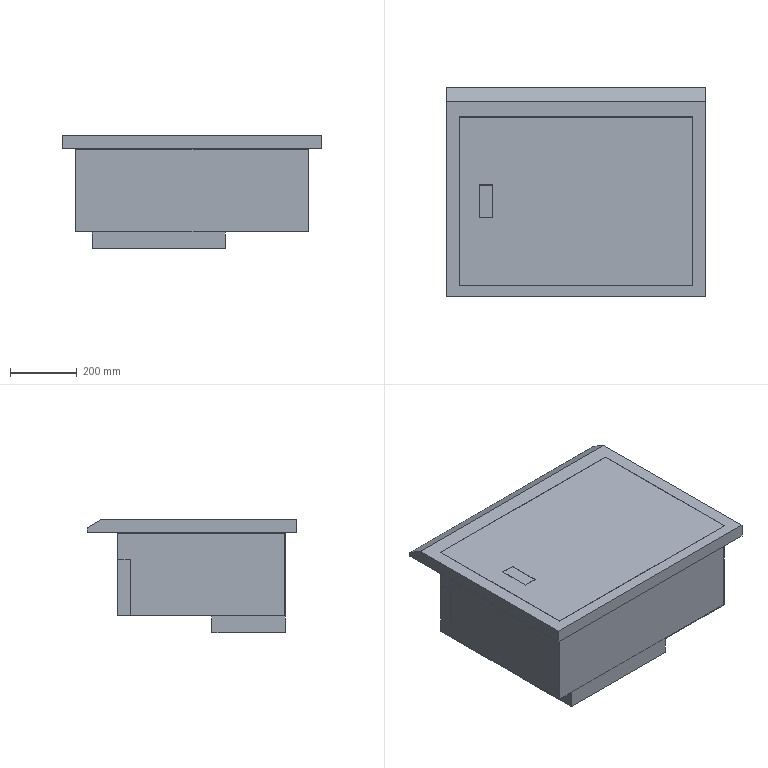Part | SolidWorks | features ICE 9, CutThin 1, Extrusion 1, Shell 1 | 1 solid | 50 faces | box 780 x 630 x 340 mm | volume 30091258 mm3 | plane 50
STEP:
#1=CARTESIAN_POINT('',(0.,505.,250.));
#2=VERTEX_POINT('',#1);
#3=CARTESIAN_POINT('',(0.,505.,0.));
#4=VERTEX_POINT('',#3);
#5=CARTESIAN_POINT('',(0.,505.,250.));
#6=DIRECTION('',(0.,0.,-1.));
#7=VECTOR('',#6,1000.);
#8=LINE('',#5,#7);
#9=EDGE_CURVE('',#2,#4,#8,.T.);
#10=ORIENTED_EDGE('',*,*,#9,.T.);
#11=CARTESIAN_POINT('',(0.,0.,0.));
#12=VERTEX_POINT('',#11);
#13=CARTESIAN_POINT('',(0.,0.,0.));
#14=DIRECTION('',(0.,-1.,0.));
#15=VECTOR('',#14,1000.);
#16=LINE('',#13,#15);
#17=EDGE_CURVE('',#4,#12,#16,.T.);
#18=ORIENTED_EDGE('',*,*,#17,.T.);
#19=CARTESIAN_POINT('',(0.,0.,250.));
#20=VERTEX_POINT('',#19);
#21=CARTESIAN_POINT('',(0.,0.,250.));
#22=DIRECTION('',(0.,0.,-1.));
#23=VECTOR('',#22,1000.);
#24=LINE('',#21,#23);
#25=EDGE_CURVE('',#20,#12,#24,.T.);
#26=ORIENTED_EDGE('',*,*,#25,.F.);
#27=CARTESIAN_POINT('',(0.,0.,250.));
#28=DIRECTION('',(0.,-1.,0.));
#29=VECTOR('',#28,1000.);
#30=LINE('',#27,#29);
#31=EDGE_CURVE('',#2,#20,#30,.T.);
#32=ORIENTED_EDGE('',*,*,#31,.F.);
#33=EDGE_LOOP('',(#10,#18,#26,#32));
#34=FACE_OUTER_BOUND('',#33,.T.);
#35=CARTESIAN_POINT('',(0.,0.,250.));
#36=DIRECTION('',(1.,0.,0.));
#37=DIRECTION('',(0.,0.,-1.));
#38=AXIS2_PLACEMENT_3D('',#35,#36,#37);
#39=PLANE('',#38);
#40=ADVANCED_FACE('',(#34),#39,.F.);
#41=ORIENTED_EDGE('',*,*,#25,.T.);
#42=CARTESIAN_POINT('',(50.,0.,0.));
#43=VERTEX_POINT('',#42);
#44=CARTESIAN_POINT('',(0.,0.,0.));
#45=DIRECTION('',(1.,0.,0.));
#46=VECTOR('',#45,1000.);
#47=LINE('',#44,#46);
#48=EDGE_CURVE('',#12,#43,#47,.T.);
#49=ORIENTED_EDGE('',*,*,#48,.T.);
#50=CARTESIAN_POINT('',(50.,0.,-50.));
#51=VERTEX_POINT('',#50);
#52=CARTESIAN_POINT('',(50.,0.,-50.));
#53=DIRECTION('',(0.,0.,1.));
#54=VECTOR('',#53,1000.);
#55=LINE('',#52,#54);
#56=EDGE_CURVE('',#51,#43,#55,.T.);
#57=ORIENTED_EDGE('',*,*,#56,.F.);
#58=CARTESIAN_POINT('',(450.,0.,-50.));
#59=VERTEX_POINT('',#58);
#60=CARTESIAN_POINT('',(50.,0.,-50.));
#61=DIRECTION('',(-1.,0.,0.));
#62=VECTOR('',#61,1000.);
#63=LINE('',#60,#62);
#64=EDGE_CURVE('',#59,#51,#63,.T.);
#65=ORIENTED_EDGE('',*,*,#64,.F.);
#66=CARTESIAN_POINT('',(450.,0.,0.));
#67=VERTEX_POINT('',#66);
#68=CARTESIAN_POINT('',(450.,0.,-50.));
#69=DIRECTION('',(0.,0.,1.));
#70=VECTOR('',#69,1000.);
#71=LINE('',#68,#70);
#72=EDGE_CURVE('',#59,#67,#71,.T.);
#73=ORIENTED_EDGE('',*,*,#72,.T.);
#74=CARTESIAN_POINT('',(700.,0.,0.));
#75=VERTEX_POINT('',#74);
#76=CARTESIAN_POINT('',(0.,0.,0.));
#77=DIRECTION('',(1.,0.,0.));
#78=VECTOR('',#77,1000.);
#79=LINE('',#76,#78);
#80=EDGE_CURVE('',#67,#75,#79,.T.);
#81=ORIENTED_EDGE('',*,*,#80,.T.);
#82=CARTESIAN_POINT('',(700.,0.,250.));
#83=VERTEX_POINT('',#82);
#84=CARTESIAN_POINT('',(700.,0.,250.));
#85=DIRECTION('',(0.,0.,-1.));
#86=VECTOR('',#85,1000.);
#87=LINE('',#84,#86);
#88=EDGE_CURVE('',#83,#75,#87,.T.);
#89=ORIENTED_EDGE('',*,*,#88,.F.);
#90=CARTESIAN_POINT('',(0.,0.,250.));
#91=DIRECTION('',(1.,0.,0.));
#92=VECTOR('',#91,1000.);
#93=LINE('',#90,#92);
#94=EDGE_CURVE('',#20,#83,#93,.T.);
#95=ORIENTED_EDGE('',*,*,#94,.F.);
#96=EDGE_LOOP('',(#41,#49,#57,#65,#73,#81,#89,#95));
#97=FACE_OUTER_BOUND('',#96,.T.);
#98=CARTESIAN_POINT('',(0.,0.,250.));
#99=DIRECTION('',(0.,1.,0.));
#100=DIRECTION('',(0.,0.,1.));
#101=AXIS2_PLACEMENT_3D('',#98,#99,#100);
#102=PLANE('',#101);
#103=ADVANCED_FACE('',(#97),#102,.F.);
#104=CARTESIAN_POINT('',(700.,505.,0.));
#105=VERTEX_POINT('',#104);
#106=CARTESIAN_POINT('',(700.,0.,0.));
#107=DIRECTION('',(0.,1.,0.));
#108=VECTOR('',#107,1000.);
#109=LINE('',#106,#108);
#110=EDGE_CURVE('',#75,#105,#109,.T.);
#111=ORIENTED_EDGE('',*,*,#110,.T.);
#112=CARTESIAN_POINT('',(700.,505.,250.));
#113=VERTEX_POINT('',#112);
#114=CARTESIAN_POINT('',(700.,505.,250.));
#115=DIRECTION('',(0.,0.,-1.));
#116=VECTOR('',#115,1000.);
#117=LINE('',#114,#116);
#118=EDGE_CURVE('',#113,#105,#117,.T.);
#119=ORIENTED_EDGE('',*,*,#118,.F.);
#120=CARTESIAN_POINT('',(700.,0.,250.));
#121=DIRECTION('',(0.,1.,0.));
#122=VECTOR('',#121,1000.);
#123=LINE('',#120,#122);
#124=EDGE_CURVE('',#83,#113,#123,.T.);
#125=ORIENTED_EDGE('',*,*,#124,.F.);
#126=ORIENTED_EDGE('',*,*,#88,.T.);
#127=EDGE_LOOP('',(#111,#119,#125,#126));
#128=FACE_OUTER_BOUND('',#127,.T.);
#129=CARTESIAN_POINT('',(700.,0.,250.));
#130=DIRECTION('',(-1.,0.,0.));
#131=DIRECTION('',(0.,0.,1.));
#132=AXIS2_PLACEMENT_3D('',#129,#130,#131);
#133=PLANE('',#132);
#134=ADVANCED_FACE('',(#128),#133,.F.);
#135=ORIENTED_EDGE('',*,*,#118,.T.);
#136=CARTESIAN_POINT('',(700.,505.,0.));
#137=DIRECTION('',(-1.,0.,0.));
#138=VECTOR('',#137,1000.);
#139=LINE('',#136,#138);
#140=EDGE_CURVE('',#105,#4,#139,.T.);
#141=ORIENTED_EDGE('',*,*,#140,.T.);
#142=ORIENTED_EDGE('',*,*,#9,.F.);
#143=CARTESIAN_POINT('',(0.,505.,250.));
#144=DIRECTION('',(-1.,0.,0.));
#145=VECTOR('',#144,1000.);
#146=LINE('',#143,#145);
#147=EDGE_CURVE('',#113,#2,#146,.T.);
#148=ORIENTED_EDGE('',*,*,#147,.F.);
#149=EDGE_LOOP('',(#135,#141,#142,#148));
#150=FACE_OUTER_BOUND('',#149,.T.);
#151=CARTESIAN_POINT('',(0.,505.,250.));
#152=DIRECTION('',(0.,-1.,0.));
#153=DIRECTION('',(0.,0.,-1.));
#154=AXIS2_PLACEMENT_3D('',#151,#152,#153);
#155=PLANE('',#154);
#156=ADVANCED_FACE('',(#150),#155,.F.);
#157=CARTESIAN_POINT('',(50.,220.,0.));
#158=VERTEX_POINT('',#157);
#159=CARTESIAN_POINT('',(50.,0.,0.));
#160=DIRECTION('',(0.,1.,0.));
#161=VECTOR('',#160,1000.);
#162=LINE('',#159,#161);
#163=EDGE_CURVE('',#43,#158,#162,.T.);
#164=ORIENTED_EDGE('',*,*,#163,.F.);
#165=ORIENTED_EDGE('',*,*,#48,.F.);
#166=ORIENTED_EDGE('',*,*,#17,.F.);
#167=ORIENTED_EDGE('',*,*,#140,.F.);
#168=ORIENTED_EDGE('',*,*,#110,.F.);
#169=ORIENTED_EDGE('',*,*,#80,.F.);
#170=CARTESIAN_POINT('',(450.,220.,0.));
#171=VERTEX_POINT('',#170);
#172=CARTESIAN_POINT('',(450.,0.,0.));
#173=DIRECTION('',(0.,-1.,0.));
#174=VECTOR('',#173,1000.);
#175=LINE('',#172,#174);
#176=EDGE_CURVE('',#171,#67,#175,.T.);
#177=ORIENTED_EDGE('',*,*,#176,.F.);
#178=CARTESIAN_POINT('',(50.,220.,0.));
#179=DIRECTION('',(1.,0.,0.));
#180=VECTOR('',#179,1000.);
#181=LINE('',#178,#180);
#182=EDGE_CURVE('',#158,#171,#181,.T.);
#183=ORIENTED_EDGE('',*,*,#182,.F.);
#184=EDGE_LOOP('',(#164,#165,#166,#167,#168,#169,#177,#183));
#185=FACE_OUTER_BOUND('',#184,.T.);
#186=CARTESIAN_POINT('',(0.,0.,0.));
#187=DIRECTION('',(0.,0.,-1.));
#188=DIRECTION('',(-1.,0.,0.));
#189=AXIS2_PLACEMENT_3D('',#186,#187,#188);
#190=PLANE('',#189);
#191=ADVANCED_FACE('',(#185),#190,.T.);
#192=ORIENTED_EDGE('',*,*,#163,.T.);
#193=CARTESIAN_POINT('',(50.,220.,-50.));
#194=VERTEX_POINT('',#193);
#195=CARTESIAN_POINT('',(50.,220.,-50.));
#196=DIRECTION('',(0.,0.,1.));
#197=VECTOR('',#196,1000.);
#198=LINE('',#195,#197);
#199=EDGE_CURVE('',#194,#158,#198,.T.);
#200=ORIENTED_EDGE('',*,*,#199,.F.);
#201=CARTESIAN_POINT('',(50.,0.,-50.));
#202=DIRECTION('',(0.,1.,0.));
#203=VECTOR('',#202,1000.);
#204=LINE('',#201,#203);
#205=EDGE_CURVE('',#51,#194,#204,.T.);
#206=ORIENTED_EDGE('',*,*,#205,.F.);
#207=ORIENTED_EDGE('',*,*,#56,.T.);
#208=EDGE_LOOP('',(#192,#200,#206,#207));
#209=FACE_OUTER_BOUND('',#208,.T.);
#210=CARTESIAN_POINT('',(50.,0.,-50.));
#211=DIRECTION('',(1.,0.,0.));
#212=DIRECTION('',(0.,1.,0.));
#213=AXIS2_PLACEMENT_3D('',#210,#211,#212);
#214=PLANE('',#213);
#215=ADVANCED_FACE('',(#209),#214,.F.);
#216=ORIENTED_EDGE('',*,*,#182,.T.);
#217=CARTESIAN_POINT('',(450.,220.,-50.));
#218=VERTEX_POINT('',#217);
#219=CARTESIAN_POINT('',(450.,220.,-50.));
#220=DIRECTION('',(0.,0.,1.));
#221=VECTOR('',#220,1000.);
#222=LINE('',#219,#221);
#223=EDGE_CURVE('',#218,#171,#222,.T.);
#224=ORIENTED_EDGE('',*,*,#223,.F.);
#225=CARTESIAN_POINT('',(50.,220.,-50.));
#226=DIRECTION('',(1.,0.,0.));
#227=VECTOR('',#226,1000.);
#228=LINE('',#225,#227);
#229=EDGE_CURVE('',#194,#218,#228,.T.);
#230=ORIENTED_EDGE('',*,*,#229,.F.);
#231=ORIENTED_EDGE('',*,*,#199,.T.);
#232=EDGE_LOOP('',(#216,#224,#230,#231));
#233=FACE_OUTER_BOUND('',#232,.T.);
#234=CARTESIAN_POINT('',(50.,220.,-50.));
#235=DIRECTION('',(0.,-1.,0.));
#236=DIRECTION('',(1.,0.,0.));
#237=AXIS2_PLACEMENT_3D('',#234,#235,#236);
#238=PLANE('',#237);
#239=ADVANCED_FACE('',(#233),#238,.F.);
#240=ORIENTED_EDGE('',*,*,#176,.T.);
#241=ORIENTED_EDGE('',*,*,#72,.F.);
#242=CARTESIAN_POINT('',(450.,0.,-50.));
#243=DIRECTION('',(0.,-1.,0.));
#244=VECTOR('',#243,1000.);
#245=LINE('',#242,#244);
#246=EDGE_CURVE('',#218,#59,#245,.T.);
#247=ORIENTED_EDGE('',*,*,#246,.F.);
#248=ORIENTED_EDGE('',*,*,#223,.T.);
#249=EDGE_LOOP('',(#240,#241,#247,#248));
#250=FACE_OUTER_BOUND('',#249,.T.);
#251=CARTESIAN_POINT('',(450.,0.,-50.));
#252=DIRECTION('',(-1.,0.,0.));
#253=DIRECTION('',(0.,-1.,0.));
#254=AXIS2_PLACEMENT_3D('',#251,#252,#253);
#255=PLANE('',#254);
#256=ADVANCED_FACE('',(#250),#255,.F.);
#257=ORIENTED_EDGE('',*,*,#205,.T.);
#258=ORIENTED_EDGE('',*,*,#229,.T.);
#259=ORIENTED_EDGE('',*,*,#246,.T.);
#260=ORIENTED_EDGE('',*,*,#64,.T.);
#261=EDGE_LOOP('',(#257,#258,#259,#260));
#262=FACE_OUTER_BOUND('',#261,.T.);
#263=CARTESIAN_POINT('',(0.,0.,-50.));
#264=DIRECTION('',(0.,0.,-1.));
#265=DIRECTION('',(-1.,0.,0.));
#266=AXIS2_PLACEMENT_3D('',#263,#264,#265);
#267=PLANE('',#266);
#268=ADVANCED_FACE('',(#262),#267,.T.);
#269=CARTESIAN_POINT('',(700.5,505.5,290.));
#270=VERTEX_POINT('',#269);
#271=CARTESIAN_POINT('',(-0.5,505.5,290.));
#272=VERTEX_POINT('',#271);
#273=CARTESIAN_POINT('',(700.,505.5,290.));
#274=DIRECTION('',(-1.,0.,0.));
#275=VECTOR('',#274,1000.);
#276=LINE('',#273,#275);
#277=EDGE_CURVE('',#270,#272,#276,.T.);
#278=ORIENTED_EDGE('',*,*,#277,.F.);
#279=CARTESIAN_POINT('',(700.5,-0.5,290.));
#280=VERTEX_POINT('',#279);
#281=CARTESIAN_POINT('',(700.5,0.,290.));
#282=DIRECTION('',(0.,1.,0.));
#283=VECTOR('',#282,1000.);
#284=LINE('',#281,#283);
#285=EDGE_CURVE('',#280,#270,#284,.T.);
#286=ORIENTED_EDGE('',*,*,#285,.F.);
#287=CARTESIAN_POINT('',(-0.5,-0.5,290.));
#288=VERTEX_POINT('',#287);
#289=CARTESIAN_POINT('',(0.,-0.5,290.));
#290=DIRECTION('',(1.,0.,0.));
#291=VECTOR('',#290,1000.);
#292=LINE('',#289,#291);
#293=EDGE_CURVE('',#288,#280,#292,.T.);
#294=ORIENTED_EDGE('',*,*,#293,.F.);
#295=CARTESIAN_POINT('',(-0.5,505.,290.));
#296=DIRECTION('',(0.,-1.,0.));
#297=VECTOR('',#296,1000.);
#298=LINE('',#295,#297);
#299=EDGE_CURVE('',#272,#288,#298,.T.);
#300=ORIENTED_EDGE('',*,*,#299,.F.);
#301=EDGE_LOOP('',(#278,#286,#294,#300));
#302=FACE_BOUND('',#301,.T.);
#303=CARTESIAN_POINT('',(740.,551.699,290.));
#304=VERTEX_POINT('',#303);
#305=CARTESIAN_POINT('',(-40.,551.699,290.));
#306=VERTEX_POINT('',#305);
#307=CARTESIAN_POINT('',(740.,551.699,290.));
#308=DIRECTION('',(-1.,0.,0.));
#309=VECTOR('',#308,1000.);
#310=LINE('',#307,#309);
#311=EDGE_CURVE('',#304,#306,#310,.T.);
#312=ORIENTED_EDGE('',*,*,#311,.T.);
#313=CARTESIAN_POINT('',(-40.,-35.,290.));
#314=VERTEX_POINT('',#313);
#315=CARTESIAN_POINT('',(-40.,595.,290.));
#316=DIRECTION('',(0.,-1.,0.));
#317=VECTOR('',#316,1000.);
#318=LINE('',#315,#317);
#319=EDGE_CURVE('',#306,#314,#318,.T.);
#320=ORIENTED_EDGE('',*,*,#319,.T.);
#321=CARTESIAN_POINT('',(740.,-35.,290.));
#322=VERTEX_POINT('',#321);
#323=CARTESIAN_POINT('',(-40.,-35.,290.));
#324=DIRECTION('',(1.,0.,0.));
#325=VECTOR('',#324,1000.);
#326=LINE('',#323,#325);
#327=EDGE_CURVE('',#314,#322,#326,.T.);
#328=ORIENTED_EDGE('',*,*,#327,.T.);
#329=CARTESIAN_POINT('',(740.,595.,290.));
#330=DIRECTION('',(0.,1.,0.));
#331=VECTOR('',#330,1000.);
#332=LINE('',#329,#331);
#333=EDGE_CURVE('',#322,#304,#332,.T.);
#334=ORIENTED_EDGE('',*,*,#333,.T.);
#335=EDGE_LOOP('',(#312,#320,#328,#334));
#336=FACE_OUTER_BOUND('',#335,.T.);
#337=CARTESIAN_POINT('',(0.,0.,290.));
#338=DIRECTION('',(0.,0.,1.));
#339=DIRECTION('',(1.,0.,0.));
#340=AXIS2_PLACEMENT_3D('',#337,#338,#339);
#341=PLANE('',#340);
#342=ADVANCED_FACE('',(#302,#336),#341,.T.);
#343=CARTESIAN_POINT('',(-40.,595.,265.));
#344=VERTEX_POINT('',#343);
#345=CARTESIAN_POINT('',(-40.,595.,250.));
#346=VERTEX_POINT('',#345);
#347=CARTESIAN_POINT('',(-40.,595.,290.));
#348=DIRECTION('',(0.,0.,-1.));
#349=VECTOR('',#348,1000.);
#350=LINE('',#347,#349);
#351=EDGE_CURVE('',#344,#346,#350,.T.);
#352=ORIENTED_EDGE('',*,*,#351,.F.);
#353=CARTESIAN_POINT('',(740.,595.,265.));
#354=VERTEX_POINT('',#353);
#355=CARTESIAN_POINT('',(740.,595.,265.));
#356=DIRECTION('',(-1.,0.,0.));
#357=VECTOR('',#356,1000.);
#358=LINE('',#355,#357);
#359=EDGE_CURVE('',#354,#344,#358,.T.);
#360=ORIENTED_EDGE('',*,*,#359,.F.);
#361=CARTESIAN_POINT('',(740.,595.,250.));
#362=VERTEX_POINT('',#361);
#363=CARTESIAN_POINT('',(740.,595.,290.));
#364=DIRECTION('',(0.,0.,-1.));
#365=VECTOR('',#364,1000.);
#366=LINE('',#363,#365);
#367=EDGE_CURVE('',#354,#362,#366,.T.);
#368=ORIENTED_EDGE('',*,*,#367,.T.);
#369=CARTESIAN_POINT('',(-40.,595.,250.));
#370=DIRECTION('',(-1.,0.,0.));
#371=VECTOR('',#370,1000.);
#372=LINE('',#369,#371);
#373=EDGE_CURVE('',#362,#346,#372,.T.);
#374=ORIENTED_EDGE('',*,*,#373,.T.);
#375=EDGE_LOOP('',(#352,#360,#368,#374));
#376=FACE_OUTER_BOUND('',#375,.T.);
#377=CARTESIAN_POINT('',(-40.,595.,290.));
#378=DIRECTION('',(0.,-1.,0.));
#379=DIRECTION('',(0.,0.,-1.));
#380=AXIS2_PLACEMENT_3D('',#377,#378,#379);
#381=PLANE('',#380);
#382=ADVANCED_FACE('',(#376),#381,.F.);
#383=ORIENTED_EDGE('',*,*,#367,.F.);
#384=CARTESIAN_POINT('',(740.,595.,265.));
#385=DIRECTION('',(0.,-0.866,0.5));
#386=VECTOR('',#385,1000.);
#387=LINE('',#384,#386);
#388=EDGE_CURVE('',#354,#304,#387,.T.);
#389=ORIENTED_EDGE('',*,*,#388,.T.);
#390=ORIENTED_EDGE('',*,*,#333,.F.);
#391=CARTESIAN_POINT('',(740.,-35.,250.));
#392=VERTEX_POINT('',#391);
#393=CARTESIAN_POINT('',(740.,-35.,290.));
#394=DIRECTION('',(0.,0.,-1.));
#395=VECTOR('',#394,1000.);
#396=LINE('',#393,#395);
#397=EDGE_CURVE('',#322,#392,#396,.T.);
#398=ORIENTED_EDGE('',*,*,#397,.T.);
#399=CARTESIAN_POINT('',(740.,595.,250.));
#400=DIRECTION('',(0.,1.,0.));
#401=VECTOR('',#400,1000.);
#402=LINE('',#399,#401);
#403=EDGE_CURVE('',#392,#362,#402,.T.);
#404=ORIENTED_EDGE('',*,*,#403,.T.);
#405=EDGE_LOOP('',(#383,#389,#390,#398,#404));
#406=FACE_OUTER_BOUND('',#405,.T.);
#407=CARTESIAN_POINT('',(740.,595.,290.));
#408=DIRECTION('',(-1.,0.,0.));
#409=DIRECTION('',(0.,-1.,0.));
#410=AXIS2_PLACEMENT_3D('',#407,#408,#409);
#411=PLANE('',#410);
#412=ADVANCED_FACE('',(#406),#411,.F.);
#413=CARTESIAN_POINT('',(-40.,-35.,250.));
#414=VERTEX_POINT('',#413);
#415=CARTESIAN_POINT('',(-40.,-35.,250.));
#416=DIRECTION('',(1.,0.,0.));
#417=VECTOR('',#416,1000.);
#418=LINE('',#415,#417);
#419=EDGE_CURVE('',#414,#392,#418,.T.);
#420=ORIENTED_EDGE('',*,*,#419,.T.);
#421=ORIENTED_EDGE('',*,*,#397,.F.);
#422=ORIENTED_EDGE('',*,*,#327,.F.);
#423=CARTESIAN_POINT('',(-40.,-35.,290.));
#424=DIRECTION('',(0.,0.,-1.));
#425=VECTOR('',#424,1000.);
#426=LINE('',#423,#425);
#427=EDGE_CURVE('',#314,#414,#426,.T.);
#428=ORIENTED_EDGE('',*,*,#427,.T.);
#429=EDGE_LOOP('',(#420,#421,#422,#428));
#430=FACE_OUTER_BOUND('',#429,.T.);
#431=CARTESIAN_POINT('',(-40.,-35.,290.));
#432=DIRECTION('',(0.,1.,0.));
#433=DIRECTION('',(0.,0.,1.));
#434=AXIS2_PLACEMENT_3D('',#431,#432,#433);
#435=PLANE('',#434);
#436=ADVANCED_FACE('',(#430),#435,.F.);
#437=ORIENTED_EDGE('',*,*,#319,.F.);
#438=CARTESIAN_POINT('',(-40.,595.,265.));
#439=DIRECTION('',(0.,-0.866,0.5));
#440=VECTOR('',#439,1000.);
#441=LINE('',#438,#440);
#442=EDGE_CURVE('',#344,#306,#441,.T.);
#443=ORIENTED_EDGE('',*,*,#442,.F.);
#444=ORIENTED_EDGE('',*,*,#351,.T.);
#445=CARTESIAN_POINT('',(-40.,595.,250.));
#446=DIRECTION('',(0.,-1.,0.));
#447=VECTOR('',#446,1000.);
#448=LINE('',#445,#447);
#449=EDGE_CURVE('',#346,#414,#448,.T.);
#450=ORIENTED_EDGE('',*,*,#449,.T.);
#451=ORIENTED_EDGE('',*,*,#427,.F.);
#452=EDGE_LOOP('',(#437,#443,#444,#450,#451));
#453=FACE_OUTER_BOUND('',#452,.T.);
#454=CARTESIAN_POINT('',(-40.,595.,290.));
#455=DIRECTION('',(1.,0.,0.));
#456=DIRECTION('',(0.,1.,0.));
#457=AXIS2_PLACEMENT_3D('',#454,#455,#456);
#458=PLANE('',#457);
#459=ADVANCED_FACE('',(#453),#458,.F.);
#460=ORIENTED_EDGE('',*,*,#449,.F.);
#461=ORIENTED_EDGE('',*,*,#373,.F.);
#462=ORIENTED_EDGE('',*,*,#403,.F.);
#463=ORIENTED_EDGE('',*,*,#419,.F.);
#464=EDGE_LOOP('',(#460,#461,#462,#463));
#465=FACE_OUTER_BOUND('',#464,.T.);
#466=ORIENTED_EDGE('',*,*,#147,.T.);
#467=ORIENTED_EDGE('',*,*,#31,.T.);
#468=ORIENTED_EDGE('',*,*,#94,.T.);
#469=ORIENTED_EDGE('',*,*,#124,.T.);
#470=EDGE_LOOP('',(#466,#467,#468,#469));
#471=FACE_BOUND('',#470,.T.);
#472=CARTESIAN_POINT('',(0.,0.,250.));
#473=DIRECTION('',(0.,0.,1.));
#474=DIRECTION('',(1.,0.,0.));
#475=AXIS2_PLACEMENT_3D('',#472,#473,#474);
#476=PLANE('',#475);
#477=ADVANCED_FACE('',(#465,#471),#476,.F.);
#478=ORIENTED_EDGE('',*,*,#442,.T.);
#479=ORIENTED_EDGE('',*,*,#311,.F.);
#480=ORIENTED_EDGE('',*,*,#388,.F.);
#481=ORIENTED_EDGE('',*,*,#359,.T.);
#482=EDGE_LOOP('',(#478,#479,#480,#481));
#483=FACE_OUTER_BOUND('',#482,.T.);
#484=CARTESIAN_POINT('',(740.,595.,265.));
#485=DIRECTION('',(0.,-0.5,-0.866));
#486=DIRECTION('',(0.,0.866,-0.5));
#487=AXIS2_PLACEMENT_3D('',#484,#485,#486);
#488=PLANE('',#487);
#489=ADVANCED_FACE('',(#483),#488,.F.);
#490=ORIENTED_EDGE('',*,*,#277,.T.);
#491=CARTESIAN_POINT('',(-0.5,505.5,280.));
#492=VERTEX_POINT('',#491);
#493=CARTESIAN_POINT('',(-0.5,505.5,280.));
#494=DIRECTION('',(0.,0.,1.));
#495=VECTOR('',#494,1000.);
#496=LINE('',#493,#495);
#497=EDGE_CURVE('',#492,#272,#496,.T.);
#498=ORIENTED_EDGE('',*,*,#497,.F.);
#499=CARTESIAN_POINT('',(700.5,505.5,280.));
#500=VERTEX_POINT('',#499);
#501=CARTESIAN_POINT('',(700.,505.5,280.));
#502=DIRECTION('',(-1.,0.,0.));
#503=VECTOR('',#502,1000.);
#504=LINE('',#501,#503);
#505=EDGE_CURVE('',#500,#492,#504,.T.);
#506=ORIENTED_EDGE('',*,*,#505,.F.);
#507=CARTESIAN_POINT('',(700.5,505.5,280.));
#508=DIRECTION('',(0.,0.,1.));
#509=VECTOR('',#508,1000.);
#510=LINE('',#507,#509);
#511=EDGE_CURVE('',#500,#270,#510,.T.);
#512=ORIENTED_EDGE('',*,*,#511,.T.);
#513=EDGE_LOOP('',(#490,#498,#506,#512));
#514=FACE_OUTER_BOUND('',#513,.T.);
#515=CARTESIAN_POINT('',(700.,505.5,280.));
#516=DIRECTION('',(0.,1.,0.));
#517=DIRECTION('',(0.,0.,1.));
#518=AXIS2_PLACEMENT_3D('',#515,#516,#517);
#519=PLANE('',#518);
#520=ADVANCED_FACE('',(#514),#519,.F.);
#521=ORIENTED_EDGE('',*,*,#285,.T.);
#522=ORIENTED_EDGE('',*,*,#511,.F.);
#523=CARTESIAN_POINT('',(700.5,-0.5,280.));
#524=VERTEX_POINT('',#523);
#525=CARTESIAN_POINT('',(700.5,0.,280.));
#526=DIRECTION('',(0.,1.,0.));
#527=VECTOR('',#526,1000.);
#528=LINE('',#525,#527);
#529=EDGE_CURVE('',#524,#500,#528,.T.);
#530=ORIENTED_EDGE('',*,*,#529,.F.);
#531=CARTESIAN_POINT('',(700.5,-0.5,280.));
#532=DIRECTION('',(0.,0.,1.));
#533=VECTOR('',#532,1000.);
#534=LINE('',#531,#533);
#535=EDGE_CURVE('',#524,#280,#534,.T.);
#536=ORIENTED_EDGE('',*,*,#535,.T.);
#537=EDGE_LOOP('',(#521,#522,#530,#536));
#538=FACE_OUTER_BOUND('',#537,.T.);
#539=CARTESIAN_POINT('',(700.5,0.,280.));
#540=DIRECTION('',(1.,0.,0.));
#541=DIRECTION('',(0.,0.,-1.));
#542=AXIS2_PLACEMENT_3D('',#539,#540,#541);
#543=PLANE('',#542);
#544=ADVANCED_FACE('',(#538),#543,.F.);
#545=ORIENTED_EDGE('',*,*,#293,.T.);
#546=ORIENTED_EDGE('',*,*,#535,.F.);
#547=CARTESIAN_POINT('',(-0.5,-0.5,280.));
#548=VERTEX_POINT('',#547);
#549=CARTESIAN_POINT('',(0.,-0.5,280.));
#550=DIRECTION('',(1.,0.,0.));
#551=VECTOR('',#550,1000.);
#552=LINE('',#549,#551);
#553=EDGE_CURVE('',#548,#524,#552,.T.);
#554=ORIENTED_EDGE('',*,*,#553,.F.);
#555=CARTESIAN_POINT('',(-0.5,-0.5,280.));
#556=DIRECTION('',(0.,0.,1.));
#557=VECTOR('',#556,1000.);
#558=LINE('',#555,#557);
#559=EDGE_CURVE('',#548,#288,#558,.T.);
#560=ORIENTED_EDGE('',*,*,#559,.T.);
#561=EDGE_LOOP('',(#545,#546,#554,#560));
#562=FACE_OUTER_BOUND('',#561,.T.);
#563=CARTESIAN_POINT('',(0.,-0.5,280.));
#564=DIRECTION('',(0.,-1.,0.));
#565=DIRECTION('',(0.,0.,-1.));
#566=AXIS2_PLACEMENT_3D('',#563,#564,#565);
#567=PLANE('',#566);
#568=ADVANCED_FACE('',(#562),#567,.F.);
#569=ORIENTED_EDGE('',*,*,#299,.T.);
#570=ORIENTED_EDGE('',*,*,#559,.F.);
#571=CARTESIAN_POINT('',(-0.5,505.,280.));
#572=DIRECTION('',(0.,-1.,0.));
#573=VECTOR('',#572,1000.);
#574=LINE('',#571,#573);
#575=EDGE_CURVE('',#492,#548,#574,.T.);
#576=ORIENTED_EDGE('',*,*,#575,.F.);
#577=ORIENTED_EDGE('',*,*,#497,.T.);
#578=EDGE_LOOP('',(#569,#570,#576,#577));
#579=FACE_OUTER_BOUND('',#578,.T.);
#580=CARTESIAN_POINT('',(-0.5,505.,280.));
#581=DIRECTION('',(-1.,0.,0.));
#582=DIRECTION('',(0.,0.,1.));
#583=AXIS2_PLACEMENT_3D('',#580,#581,#582);
#584=PLANE('',#583);
#585=ADVANCED_FACE('',(#579),#584,.F.);
#586=CARTESIAN_POINT('',(700.,0.,280.));
#587=VERTEX_POINT('',#586);
#588=CARTESIAN_POINT('',(700.,505.,280.));
#589=VERTEX_POINT('',#588);
#590=CARTESIAN_POINT('',(700.,0.,280.));
#591=DIRECTION('',(0.,1.,0.));
#592=VECTOR('',#591,1000.);
#593=LINE('',#590,#592);
#594=EDGE_CURVE('',#587,#589,#593,.T.);
#595=ORIENTED_EDGE('',*,*,#594,.F.);
#596=CARTESIAN_POINT('',(0.,0.,280.));
#597=VERTEX_POINT('',#596);
#598=CARTESIAN_POINT('',(0.,0.,280.));
#599=DIRECTION('',(1.,0.,0.));
#600=VECTOR('',#599,1000.);
#601=LINE('',#598,#600);
#602=EDGE_CURVE('',#597,#587,#601,.T.);
#603=ORIENTED_EDGE('',*,*,#602,.F.);
#604=CARTESIAN_POINT('',(0.,505.,280.));
#605=VERTEX_POINT('',#604);
#606=CARTESIAN_POINT('',(0.,505.,280.));
#607=DIRECTION('',(0.,-1.,0.));
#608=VECTOR('',#607,1000.);
#609=LINE('',#606,#608);
#610=EDGE_CURVE('',#605,#597,#609,.T.);
#611=ORIENTED_EDGE('',*,*,#610,.F.);
#612=CARTESIAN_POINT('',(700.,505.,280.));
#613=DIRECTION('',(-1.,0.,0.));
#614=VECTOR('',#613,1000.);
#615=LINE('',#612,#614);
#616=EDGE_CURVE('',#589,#605,#615,.T.);
#617=ORIENTED_EDGE('',*,*,#616,.F.);
#618=EDGE_LOOP('',(#595,#603,#611,#617));
#619=FACE_BOUND('',#618,.T.);
#620=ORIENTED_EDGE('',*,*,#505,.T.);
#621=ORIENTED_EDGE('',*,*,#575,.T.);
#622=ORIENTED_EDGE('',*,*,#553,.T.);
#623=ORIENTED_EDGE('',*,*,#529,.T.);
#624=EDGE_LOOP('',(#620,#621,#622,#623));
#625=FACE_OUTER_BOUND('',#624,.T.);
#626=CARTESIAN_POINT('',(0.,0.,280.));
#627=DIRECTION('',(0.,0.,1.));
#628=DIRECTION('',(1.,0.,0.));
#629=AXIS2_PLACEMENT_3D('',#626,#627,#628);
#630=PLANE('',#629);
#631=ADVANCED_FACE('',(#619,#625),#630,.T.);
#632=CARTESIAN_POINT('',(700.,505.,290.));
#633=VERTEX_POINT('',#632);
#634=CARTESIAN_POINT('',(0.,505.,290.));
#635=VERTEX_POINT('',#634);
#636=CARTESIAN_POINT('',(700.,505.,290.));
#637=DIRECTION('',(-1.,0.,0.));
#638=VECTOR('',#637,1000.);
#639=LINE('',#636,#638);
#640=EDGE_CURVE('',#633,#635,#639,.T.);
#641=ORIENTED_EDGE('',*,*,#640,.F.);
#642=CARTESIAN_POINT('',(700.,505.,280.));
#643=DIRECTION('',(0.,0.,1.));
#644=VECTOR('',#643,1000.);
#645=LINE('',#642,#644);
#646=EDGE_CURVE('',#589,#633,#645,.T.);
#647=ORIENTED_EDGE('',*,*,#646,.F.);
#648=ORIENTED_EDGE('',*,*,#616,.T.);
#649=CARTESIAN_POINT('',(0.,505.,280.));
#650=DIRECTION('',(0.,0.,1.));
#651=VECTOR('',#650,1000.);
#652=LINE('',#649,#651);
#653=EDGE_CURVE('',#605,#635,#652,.T.);
#654=ORIENTED_EDGE('',*,*,#653,.T.);
#655=EDGE_LOOP('',(#641,#647,#648,#654));
#656=FACE_OUTER_BOUND('',#655,.T.);
#657=CARTESIAN_POINT('',(700.,505.,280.));
#658=DIRECTION('',(0.,1.,0.));
#659=DIRECTION('',(0.,0.,1.));
#660=AXIS2_PLACEMENT_3D('',#657,#658,#659);
#661=PLANE('',#660);
#662=ADVANCED_FACE('',(#656),#661,.T.);
#663=CARTESIAN_POINT('',(700.,0.,290.));
#664=VERTEX_POINT('',#663);
#665=CARTESIAN_POINT('',(700.,0.,290.));
#666=DIRECTION('',(0.,1.,0.));
#667=VECTOR('',#666,1000.);
#668=LINE('',#665,#667);
#669=EDGE_CURVE('',#664,#633,#668,.T.);
#670=ORIENTED_EDGE('',*,*,#669,.F.);
#671=CARTESIAN_POINT('',(700.,0.,280.));
#672=DIRECTION('',(0.,0.,1.));
#673=VECTOR('',#672,1000.);
#674=LINE('',#671,#673);
#675=EDGE_CURVE('',#587,#664,#674,.T.);
#676=ORIENTED_EDGE('',*,*,#675,.F.);
#677=ORIENTED_EDGE('',*,*,#594,.T.);
#678=ORIENTED_EDGE('',*,*,#646,.T.);
#679=EDGE_LOOP('',(#670,#676,#677,#678));
#680=FACE_OUTER_BOUND('',#679,.T.);
#681=CARTESIAN_POINT('',(700.,0.,280.));
#682=DIRECTION('',(1.,0.,0.));
#683=DIRECTION('',(0.,0.,-1.));
#684=AXIS2_PLACEMENT_3D('',#681,#682,#683);
#685=PLANE('',#684);
#686=ADVANCED_FACE('',(#680),#685,.T.);
#687=CARTESIAN_POINT('',(0.,0.,290.));
#688=VERTEX_POINT('',#687);
#689=CARTESIAN_POINT('',(0.,0.,290.));
#690=DIRECTION('',(1.,0.,0.));
#691=VECTOR('',#690,1000.);
#692=LINE('',#689,#691);
#693=EDGE_CURVE('',#688,#664,#692,.T.);
#694=ORIENTED_EDGE('',*,*,#693,.F.);
#695=CARTESIAN_POINT('',(0.,0.,280.));
#696=DIRECTION('',(0.,0.,1.));
#697=VECTOR('',#696,1000.);
#698=LINE('',#695,#697);
#699=EDGE_CURVE('',#597,#688,#698,.T.);
#700=ORIENTED_EDGE('',*,*,#699,.F.);
#701=ORIENTED_EDGE('',*,*,#602,.T.);
#702=ORIENTED_EDGE('',*,*,#675,.T.);
#703=EDGE_LOOP('',(#694,#700,#701,#702));
#704=FACE_OUTER_BOUND('',#703,.T.);
#705=CARTESIAN_POINT('',(0.,0.,280.));
#706=DIRECTION('',(0.,-1.,0.));
#707=DIRECTION('',(0.,0.,-1.));
#708=AXIS2_PLACEMENT_3D('',#705,#706,#707);
#709=PLANE('',#708);
#710=ADVANCED_FACE('',(#704),#709,.T.);
#711=CARTESIAN_POINT('',(0.,505.,290.));
#712=DIRECTION('',(0.,-1.,0.));
#713=VECTOR('',#712,1000.);
#714=LINE('',#711,#713);
#715=EDGE_CURVE('',#635,#688,#714,.T.);
#716=ORIENTED_EDGE('',*,*,#715,.F.);
#717=ORIENTED_EDGE('',*,*,#653,.F.);
#718=ORIENTED_EDGE('',*,*,#610,.T.);
#719=ORIENTED_EDGE('',*,*,#699,.T.);
#720=EDGE_LOOP('',(#716,#717,#718,#719));
#721=FACE_OUTER_BOUND('',#720,.T.);
#722=CARTESIAN_POINT('',(0.,505.,280.));
#723=DIRECTION('',(-1.,0.,0.));
#724=DIRECTION('',(0.,0.,1.));
#725=AXIS2_PLACEMENT_3D('',#722,#723,#724);
#726=PLANE('',#725);
#727=ADVANCED_FACE('',(#721),#726,.T.);
#728=CARTESIAN_POINT('',(59.5,301.,290.));
#729=VERTEX_POINT('',#728);
#730=CARTESIAN_POINT('',(59.5,204.,290.));
#731=VERTEX_POINT('',#730);
#732=CARTESIAN_POINT('',(59.5,300.5,290.));
#733=DIRECTION('',(0.,-1.,0.));
#734=VECTOR('',#733,1000.);
#735=LINE('',#732,#734);
#736=EDGE_CURVE('',#729,#731,#735,.T.);
#737=ORIENTED_EDGE('',*,*,#736,.F.);
#738=CARTESIAN_POINT('',(100.5,301.,290.));
#739=VERTEX_POINT('',#738);
#740=CARTESIAN_POINT('',(60.,301.,290.));
#741=DIRECTION('',(-1.,0.,0.));
#742=VECTOR('',#741,1000.);
#743=LINE('',#740,#742);
#744=EDGE_CURVE('',#739,#729,#743,.T.);
#745=ORIENTED_EDGE('',*,*,#744,.F.);
#746=CARTESIAN_POINT('',(100.5,204.,290.));
#747=VERTEX_POINT('',#746);
#748=CARTESIAN_POINT('',(100.5,300.5,290.));
#749=DIRECTION('',(0.,1.,0.));
#750=VECTOR('',#749,1000.);
#751=LINE('',#748,#750);
#752=EDGE_CURVE('',#747,#739,#751,.T.);
#753=ORIENTED_EDGE('',*,*,#752,.F.);
#754=CARTESIAN_POINT('',(60.,204.,290.));
#755=DIRECTION('',(1.,0.,0.));
#756=VECTOR('',#755,1000.);
#757=LINE('',#754,#756);
#758=EDGE_CURVE('',#731,#747,#757,.T.);
#759=ORIENTED_EDGE('',*,*,#758,.F.);
#760=EDGE_LOOP('',(#737,#745,#753,#759));
#761=FACE_BOUND('',#760,.T.);
#762=ORIENTED_EDGE('',*,*,#669,.T.);
#763=ORIENTED_EDGE('',*,*,#640,.T.);
#764=ORIENTED_EDGE('',*,*,#715,.T.);
#765=ORIENTED_EDGE('',*,*,#693,.T.);
#766=EDGE_LOOP('',(#762,#763,#764,#765));
#767=FACE_OUTER_BOUND('',#766,.T.);
#768=CARTESIAN_POINT('',(0.,0.,290.));
#769=DIRECTION('',(0.,0.,1.));
#770=DIRECTION('',(1.,0.,0.));
#771=AXIS2_PLACEMENT_3D('',#768,#769,#770);
#772=PLANE('',#771);
#773=ADVANCED_FACE('',(#761,#767),#772,.T.);
#774=ORIENTED_EDGE('',*,*,#736,.T.);
#775=CARTESIAN_POINT('',(59.5,204.,280.));
#776=VERTEX_POINT('',#775);
#777=CARTESIAN_POINT('',(59.5,204.,280.));
#778=DIRECTION('',(0.,0.,1.));
#779=VECTOR('',#778,1000.);
#780=LINE('',#777,#779);
#781=EDGE_CURVE('',#776,#731,#780,.T.);
#782=ORIENTED_EDGE('',*,*,#781,.F.);
#783=CARTESIAN_POINT('',(59.5,301.,280.));
#784=VERTEX_POINT('',#783);
#785=CARTESIAN_POINT('',(59.5,300.5,280.));
#786=DIRECTION('',(0.,-1.,0.));
#787=VECTOR('',#786,1000.);
#788=LINE('',#785,#787);
#789=EDGE_CURVE('',#784,#776,#788,.T.);
#790=ORIENTED_EDGE('',*,*,#789,.F.);
#791=CARTESIAN_POINT('',(59.5,301.,280.));
#792=DIRECTION('',(0.,0.,1.));
#793=VECTOR('',#792,1000.);
#794=LINE('',#791,#793);
#795=EDGE_CURVE('',#784,#729,#794,.T.);
#796=ORIENTED_EDGE('',*,*,#795,.T.);
#797=EDGE_LOOP('',(#774,#782,#790,#796));
#798=FACE_OUTER_BOUND('',#797,.T.);
#799=CARTESIAN_POINT('',(59.5,300.5,280.));
#800=DIRECTION('',(-1.,0.,0.));
#801=DIRECTION('',(0.,0.,1.));
#802=AXIS2_PLACEMENT_3D('',#799,#800,#801);
#803=PLANE('',#802);
#804=ADVANCED_FACE('',(#798),#803,.F.);
#805=ORIENTED_EDGE('',*,*,#744,.T.);
#806=ORIENTED_EDGE('',*,*,#795,.F.);
#807=CARTESIAN_POINT('',(100.5,301.,280.));
#808=VERTEX_POINT('',#807);
#809=CARTESIAN_POINT('',(60.,301.,280.));
#810=DIRECTION('',(-1.,0.,0.));
#811=VECTOR('',#810,1000.);
#812=LINE('',#809,#811);
#813=EDGE_CURVE('',#808,#784,#812,.T.);
#814=ORIENTED_EDGE('',*,*,#813,.F.);
#815=CARTESIAN_POINT('',(100.5,301.,280.));
#816=DIRECTION('',(0.,0.,1.));
#817=VECTOR('',#816,1000.);
#818=LINE('',#815,#817);
#819=EDGE_CURVE('',#808,#739,#818,.T.);
#820=ORIENTED_EDGE('',*,*,#819,.T.);
#821=EDGE_LOOP('',(#805,#806,#814,#820));
#822=FACE_OUTER_BOUND('',#821,.T.);
#823=CARTESIAN_POINT('',(60.,301.,280.));
#824=DIRECTION('',(0.,1.,0.));
#825=DIRECTION('',(0.,0.,1.));
#826=AXIS2_PLACEMENT_3D('',#823,#824,#825);
#827=PLANE('',#826);
#828=ADVANCED_FACE('',(#822),#827,.F.);
#829=ORIENTED_EDGE('',*,*,#752,.T.);
#830=ORIENTED_EDGE('',*,*,#819,.F.);
#831=CARTESIAN_POINT('',(100.5,204.,280.));
#832=VERTEX_POINT('',#831);
#833=CARTESIAN_POINT('',(100.5,300.5,280.));
#834=DIRECTION('',(0.,1.,0.));
#835=VECTOR('',#834,1000.);
#836=LINE('',#833,#835);
#837=EDGE_CURVE('',#832,#808,#836,.T.);
#838=ORIENTED_EDGE('',*,*,#837,.F.);
#839=CARTESIAN_POINT('',(100.5,204.,280.));
#840=DIRECTION('',(0.,0.,1.));
#841=VECTOR('',#840,1000.);
#842=LINE('',#839,#841);
#843=EDGE_CURVE('',#832,#747,#842,.T.);
#844=ORIENTED_EDGE('',*,*,#843,.T.);
#845=EDGE_LOOP('',(#829,#830,#838,#844));
#846=FACE_OUTER_BOUND('',#845,.T.);
#847=CARTESIAN_POINT('',(100.5,300.5,280.));
#848=DIRECTION('',(1.,0.,0.));
#849=DIRECTION('',(0.,0.,-1.));
#850=AXIS2_PLACEMENT_3D('',#847,#848,#849);
#851=PLANE('',#850);
#852=ADVANCED_FACE('',(#846),#851,.F.);
#853=ORIENTED_EDGE('',*,*,#758,.T.);
#854=ORIENTED_EDGE('',*,*,#843,.F.);
#855=CARTESIAN_POINT('',(60.,204.,280.));
#856=DIRECTION('',(1.,0.,0.));
#857=VECTOR('',#856,1000.);
#858=LINE('',#855,#857);
#859=EDGE_CURVE('',#776,#832,#858,.T.);
#860=ORIENTED_EDGE('',*,*,#859,.F.);
#861=ORIENTED_EDGE('',*,*,#781,.T.);
#862=EDGE_LOOP('',(#853,#854,#860,#861));
#863=FACE_OUTER_BOUND('',#862,.T.);
#864=CARTESIAN_POINT('',(60.,204.,280.));
#865=DIRECTION('',(0.,-1.,0.));
#866=DIRECTION('',(0.,0.,-1.));
#867=AXIS2_PLACEMENT_3D('',#864,#865,#866);
#868=PLANE('',#867);
#869=ADVANCED_FACE('',(#863),#868,.F.);
#870=CARTESIAN_POINT('',(100.,300.5,280.));
#871=VERTEX_POINT('',#870);
#872=CARTESIAN_POINT('',(60.,300.5,280.));
#873=VERTEX_POINT('',#872);
#874=CARTESIAN_POINT('',(60.,300.5,280.));
#875=DIRECTION('',(-1.,0.,0.));
#876=VECTOR('',#875,1000.);
#877=LINE('',#874,#876);
#878=EDGE_CURVE('',#871,#873,#877,.T.);
#879=ORIENTED_EDGE('',*,*,#878,.F.);
#880=CARTESIAN_POINT('',(100.,204.5,280.));
#881=VERTEX_POINT('',#880);
#882=CARTESIAN_POINT('',(100.,300.5,280.));
#883=DIRECTION('',(0.,1.,0.));
#884=VECTOR('',#883,1000.);
#885=LINE('',#882,#884);
#886=EDGE_CURVE('',#881,#871,#885,.T.);
#887=ORIENTED_EDGE('',*,*,#886,.F.);
#888=CARTESIAN_POINT('',(60.,204.5,280.));
#889=VERTEX_POINT('',#888);
#890=CARTESIAN_POINT('',(60.,204.5,280.));
#891=DIRECTION('',(1.,0.,0.));
#892=VECTOR('',#891,1000.);
#893=LINE('',#890,#892);
#894=EDGE_CURVE('',#889,#881,#893,.T.);
#895=ORIENTED_EDGE('',*,*,#894,.F.);
#896=CARTESIAN_POINT('',(60.,300.5,280.));
#897=DIRECTION('',(0.,-1.,0.));
#898=VECTOR('',#897,1000.);
#899=LINE('',#896,#898);
#900=EDGE_CURVE('',#873,#889,#899,.T.);
#901=ORIENTED_EDGE('',*,*,#900,.F.);
#902=EDGE_LOOP('',(#879,#887,#895,#901));
#903=FACE_BOUND('',#902,.T.);
#904=ORIENTED_EDGE('',*,*,#789,.T.);
#905=ORIENTED_EDGE('',*,*,#859,.T.);
#906=ORIENTED_EDGE('',*,*,#837,.T.);
#907=ORIENTED_EDGE('',*,*,#813,.T.);
#908=EDGE_LOOP('',(#904,#905,#906,#907));
#909=FACE_OUTER_BOUND('',#908,.T.);
#910=CARTESIAN_POINT('',(0.,0.,280.));
#911=DIRECTION('',(0.,0.,1.));
#912=DIRECTION('',(1.,0.,0.));
#913=AXIS2_PLACEMENT_3D('',#910,#911,#912);
#914=PLANE('',#913);
#915=ADVANCED_FACE('',(#903,#909),#914,.T.);
#916=CARTESIAN_POINT('',(60.,300.5,290.));
#917=VERTEX_POINT('',#916);
#918=CARTESIAN_POINT('',(60.,204.5,290.));
#919=VERTEX_POINT('',#918);
#920=CARTESIAN_POINT('',(60.,300.5,290.));
#921=DIRECTION('',(0.,-1.,0.));
#922=VECTOR('',#921,1000.);
#923=LINE('',#920,#922);
#924=EDGE_CURVE('',#917,#919,#923,.T.);
#925=ORIENTED_EDGE('',*,*,#924,.F.);
#926=CARTESIAN_POINT('',(60.,300.5,280.));
#927=DIRECTION('',(0.,0.,1.));
#928=VECTOR('',#927,1000.);
#929=LINE('',#926,#928);
#930=EDGE_CURVE('',#873,#917,#929,.T.);
#931=ORIENTED_EDGE('',*,*,#930,.F.);
#932=ORIENTED_EDGE('',*,*,#900,.T.);
#933=CARTESIAN_POINT('',(60.,204.5,280.));
#934=DIRECTION('',(0.,0.,1.));
#935=VECTOR('',#934,1000.);
#936=LINE('',#933,#935);
#937=EDGE_CURVE('',#889,#919,#936,.T.);
#938=ORIENTED_EDGE('',*,*,#937,.T.);
#939=EDGE_LOOP('',(#925,#931,#932,#938));
#940=FACE_OUTER_BOUND('',#939,.T.);
#941=CARTESIAN_POINT('',(60.,300.5,280.));
#942=DIRECTION('',(-1.,0.,0.));
#943=DIRECTION('',(0.,0.,1.));
#944=AXIS2_PLACEMENT_3D('',#941,#942,#943);
#945=PLANE('',#944);
#946=ADVANCED_FACE('',(#940),#945,.T.);
#947=CARTESIAN_POINT('',(100.,300.5,290.));
#948=VERTEX_POINT('',#947);
#949=CARTESIAN_POINT('',(60.,300.5,290.));
#950=DIRECTION('',(-1.,0.,0.));
#951=VECTOR('',#950,1000.);
#952=LINE('',#949,#951);
#953=EDGE_CURVE('',#948,#917,#952,.T.);
#954=ORIENTED_EDGE('',*,*,#953,.F.);
#955=CARTESIAN_POINT('',(100.,300.5,280.));
#956=DIRECTION('',(0.,0.,1.));
#957=VECTOR('',#956,1000.);
#958=LINE('',#955,#957);
#959=EDGE_CURVE('',#871,#948,#958,.T.);
#960=ORIENTED_EDGE('',*,*,#959,.F.);
#961=ORIENTED_EDGE('',*,*,#878,.T.);
#962=ORIENTED_EDGE('',*,*,#930,.T.);
#963=EDGE_LOOP('',(#954,#960,#961,#962));
#964=FACE_OUTER_BOUND('',#963,.T.);
#965=CARTESIAN_POINT('',(60.,300.5,280.));
#966=DIRECTION('',(0.,1.,0.));
#967=DIRECTION('',(0.,0.,1.));
#968=AXIS2_PLACEMENT_3D('',#965,#966,#967);
#969=PLANE('',#968);
#970=ADVANCED_FACE('',(#964),#969,.T.);
#971=CARTESIAN_POINT('',(100.,204.5,290.));
#972=VERTEX_POINT('',#971);
#973=CARTESIAN_POINT('',(100.,300.5,290.));
#974=DIRECTION('',(0.,1.,0.));
#975=VECTOR('',#974,1000.);
#976=LINE('',#973,#975);
#977=EDGE_CURVE('',#972,#948,#976,.T.);
#978=ORIENTED_EDGE('',*,*,#977,.F.);
#979=CARTESIAN_POINT('',(100.,204.5,280.));
#980=DIRECTION('',(0.,0.,1.));
#981=VECTOR('',#980,1000.);
#982=LINE('',#979,#981);
#983=EDGE_CURVE('',#881,#972,#982,.T.);
#984=ORIENTED_EDGE('',*,*,#983,.F.);
#985=ORIENTED_EDGE('',*,*,#886,.T.);
#986=ORIENTED_EDGE('',*,*,#959,.T.);
#987=EDGE_LOOP('',(#978,#984,#985,#986));
#988=FACE_OUTER_BOUND('',#987,.T.);
#989=CARTESIAN_POINT('',(100.,300.5,280.));
#990=DIRECTION('',(1.,0.,0.));
#991=DIRECTION('',(0.,0.,-1.));
#992=AXIS2_PLACEMENT_3D('',#989,#990,#991);
#993=PLANE('',#992);
#994=ADVANCED_FACE('',(#988),#993,.T.);
#995=CARTESIAN_POINT('',(60.,204.5,290.));
#996=DIRECTION('',(1.,0.,0.));
#997=VECTOR('',#996,1000.);
#998=LINE('',#995,#997);
#999=EDGE_CURVE('',#919,#972,#998,.T.);
#1000=ORIENTED_EDGE('',*,*,#999,.F.);
#1001=ORIENTED_EDGE('',*,*,#937,.F.);
#1002=ORIENTED_EDGE('',*,*,#894,.T.);
#1003=ORIENTED_EDGE('',*,*,#983,.T.);
#1004=EDGE_LOOP('',(#1000,#1001,#1002,#1003));
#1005=FACE_OUTER_BOUND('',#1004,.T.);
#1006=CARTESIAN_POINT('',(60.,204.5,280.));
#1007=DIRECTION('',(0.,-1.,0.));
#1008=DIRECTION('',(0.,0.,-1.));
#1009=AXIS2_PLACEMENT_3D('',#1006,#1007,#1008);
#1010=PLANE('',#1009);
#1011=ADVANCED_FACE('',(#1005),#1010,.T.);
#1012=ORIENTED_EDGE('',*,*,#953,.T.);
#1013=ORIENTED_EDGE('',*,*,#924,.T.);
#1014=ORIENTED_EDGE('',*,*,#999,.T.);
#1015=ORIENTED_EDGE('',*,*,#977,.T.);
#1016=EDGE_LOOP('',(#1012,#1013,#1014,#1015));
#1017=FACE_OUTER_BOUND('',#1016,.T.);
#1018=CARTESIAN_POINT('',(0.,0.,290.));
#1019=DIRECTION('',(0.,0.,1.));
#1020=DIRECTION('',(1.,0.,0.));
#1021=AXIS2_PLACEMENT_3D('',#1018,#1019,#1020);
#1022=PLANE('',#1021);
#1023=ADVANCED_FACE('',(#1017),#1022,.T.);
#1024=CLOSED_SHELL('',(#40,#103,#134,#156,#191,#215,#239,#256,#268,#342,#382,#412,#436,#459,#477,#489,#520,#544,#568,#585,#631,#662,#686,#710,#727,#773,#804,#828,#852,#869,#915,#946,#970,#994,#1011,#1023));
#1025=CARTESIAN_POINT('',(30.,300.5,249.5));
#1026=VERTEX_POINT('',#1025);
#1027=CARTESIAN_POINT('',(30.,204.5,249.5));
#1028=VERTEX_POINT('',#1027);
#1029=CARTESIAN_POINT('',(30.,300.5,249.5));
#1030=DIRECTION('',(0.,-1.,0.));
#1031=VECTOR('',#1030,1000.);
#1032=LINE('',#1029,#1031);
#1033=EDGE_CURVE('',#1026,#1028,#1032,.T.);
#1034=ORIENTED_EDGE('',*,*,#1033,.T.);
#1035=CARTESIAN_POINT('',(70.,204.5,249.5));
#1036=VERTEX_POINT('',#1035);
#1037=CARTESIAN_POINT('',(30.,204.5,249.5));
#1038=DIRECTION('',(1.,0.,0.));
#1039=VECTOR('',#1038,1000.);
#1040=LINE('',#1037,#1039);
#1041=EDGE_CURVE('',#1028,#1036,#1040,.T.);
#1042=ORIENTED_EDGE('',*,*,#1041,.T.);
#1043=CARTESIAN_POINT('',(70.,300.5,249.5));
#1044=VERTEX_POINT('',#1043);
#1045=CARTESIAN_POINT('',(70.,300.5,249.5));
#1046=DIRECTION('',(0.,1.,0.));
#1047=VECTOR('',#1046,1000.);
#1048=LINE('',#1045,#1047);
#1049=EDGE_CURVE('',#1036,#1044,#1048,.T.);
#1050=ORIENTED_EDGE('',*,*,#1049,.T.);
#1051=CARTESIAN_POINT('',(30.,300.5,249.5));
#1052=DIRECTION('',(-1.,0.,0.));
#1053=VECTOR('',#1052,1000.);
#1054=LINE('',#1051,#1053);
#1055=EDGE_CURVE('',#1044,#1026,#1054,.T.);
#1056=ORIENTED_EDGE('',*,*,#1055,.T.);
#1057=EDGE_LOOP('',(#1034,#1042,#1050,#1056));
#1058=FACE_OUTER_BOUND('',#1057,.T.);
#1059=CARTESIAN_POINT('',(0.,0.,249.5));
#1060=DIRECTION('',(0.,0.,1.));
#1061=DIRECTION('',(1.,0.,0.));
#1062=AXIS2_PLACEMENT_3D('',#1059,#1060,#1061);
#1063=PLANE('',#1062);
#1064=ADVANCED_FACE('',(#1058),#1063,.T.);
#1065=CARTESIAN_POINT('',(70.,204.5,250.));
#1066=VERTEX_POINT('',#1065);
#1067=CARTESIAN_POINT('',(70.,300.5,250.));
#1068=VERTEX_POINT('',#1067);
#1069=CARTESIAN_POINT('',(70.,300.5,250.));
#1070=DIRECTION('',(0.,1.,0.));
#1071=VECTOR('',#1070,1000.);
#1072=LINE('',#1069,#1071);
#1073=EDGE_CURVE('',#1066,#1068,#1072,.T.);
#1074=ORIENTED_EDGE('',*,*,#1073,.T.);
#1075=CARTESIAN_POINT('',(70.,300.5,249.5));
#1076=DIRECTION('',(0.,0.,1.));
#1077=VECTOR('',#1076,1000.);
#1078=LINE('',#1075,#1077);
#1079=EDGE_CURVE('',#1044,#1068,#1078,.T.);
#1080=ORIENTED_EDGE('',*,*,#1079,.F.);
#1081=ORIENTED_EDGE('',*,*,#1049,.F.);
#1082=CARTESIAN_POINT('',(70.,204.5,249.5));
#1083=DIRECTION('',(0.,0.,1.));
#1084=VECTOR('',#1083,1000.);
#1085=LINE('',#1082,#1084);
#1086=EDGE_CURVE('',#1036,#1066,#1085,.T.);
#1087=ORIENTED_EDGE('',*,*,#1086,.T.);
#1088=EDGE_LOOP('',(#1074,#1080,#1081,#1087));
#1089=FACE_OUTER_BOUND('',#1088,.T.);
#1090=CARTESIAN_POINT('',(70.,300.5,249.5));
#1091=DIRECTION('',(1.,0.,0.));
#1092=DIRECTION('',(0.,1.,0.));
#1093=AXIS2_PLACEMENT_3D('',#1090,#1091,#1092);
#1094=PLANE('',#1093);
#1095=ADVANCED_FACE('',(#1089),#1094,.F.);
#1096=CARTESIAN_POINT('',(30.,300.5,250.));
#1097=VERTEX_POINT('',#1096);
#1098=CARTESIAN_POINT('',(30.,300.5,250.));
#1099=DIRECTION('',(-1.,0.,0.));
#1100=VECTOR('',#1099,1000.);
#1101=LINE('',#1098,#1100);
#1102=EDGE_CURVE('',#1068,#1097,#1101,.T.);
#1103=ORIENTED_EDGE('',*,*,#1102,.T.);
#1104=CARTESIAN_POINT('',(30.,300.5,249.5));
#1105=DIRECTION('',(0.,0.,1.));
#1106=VECTOR('',#1105,1000.);
#1107=LINE('',#1104,#1106);
#1108=EDGE_CURVE('',#1026,#1097,#1107,.T.);
#1109=ORIENTED_EDGE('',*,*,#1108,.F.);
#1110=ORIENTED_EDGE('',*,*,#1055,.F.);
#1111=ORIENTED_EDGE('',*,*,#1079,.T.);
#1112=EDGE_LOOP('',(#1103,#1109,#1110,#1111));
#1113=FACE_OUTER_BOUND('',#1112,.T.);
#1114=CARTESIAN_POINT('',(30.,300.5,249.5));
#1115=DIRECTION('',(0.,1.,0.));
#1116=DIRECTION('',(0.,0.,1.));
#1117=AXIS2_PLACEMENT_3D('',#1114,#1115,#1116);
#1118=PLANE('',#1117);
#1119=ADVANCED_FACE('',(#1113),#1118,.F.);
#1120=CARTESIAN_POINT('',(30.,204.5,250.));
#1121=VERTEX_POINT('',#1120);
#1122=CARTESIAN_POINT('',(30.,300.5,250.));
#1123=DIRECTION('',(0.,-1.,0.));
#1124=VECTOR('',#1123,1000.);
#1125=LINE('',#1122,#1124);
#1126=EDGE_CURVE('',#1097,#1121,#1125,.T.);
#1127=ORIENTED_EDGE('',*,*,#1126,.T.);
#1128=CARTESIAN_POINT('',(30.,204.5,249.5));
#1129=DIRECTION('',(0.,0.,1.));
#1130=VECTOR('',#1129,1000.);
#1131=LINE('',#1128,#1130);
#1132=EDGE_CURVE('',#1028,#1121,#1131,.T.);
#1133=ORIENTED_EDGE('',*,*,#1132,.F.);
#1134=ORIENTED_EDGE('',*,*,#1033,.F.);
#1135=ORIENTED_EDGE('',*,*,#1108,.T.);
#1136=EDGE_LOOP('',(#1127,#1133,#1134,#1135));
#1137=FACE_OUTER_BOUND('',#1136,.T.);
#1138=CARTESIAN_POINT('',(30.,300.5,249.5));
#1139=DIRECTION('',(-1.,0.,0.));
#1140=DIRECTION('',(0.,0.,1.));
#1141=AXIS2_PLACEMENT_3D('',#1138,#1139,#1140);
#1142=PLANE('',#1141);
#1143=ADVANCED_FACE('',(#1137),#1142,.F.);
#1144=CARTESIAN_POINT('',(30.,204.5,250.));
#1145=DIRECTION('',(1.,0.,0.));
#1146=VECTOR('',#1145,1000.);
#1147=LINE('',#1144,#1146);
#1148=EDGE_CURVE('',#1121,#1066,#1147,.T.);
#1149=ORIENTED_EDGE('',*,*,#1148,.T.);
#1150=ORIENTED_EDGE('',*,*,#1086,.F.);
#1151=ORIENTED_EDGE('',*,*,#1041,.F.);
#1152=ORIENTED_EDGE('',*,*,#1132,.T.);
#1153=EDGE_LOOP('',(#1149,#1150,#1151,#1152));
#1154=FACE_OUTER_BOUND('',#1153,.T.);
#1155=CARTESIAN_POINT('',(30.,204.5,249.5));
#1156=DIRECTION('',(0.,-1.,0.));
#1157=DIRECTION('',(0.,0.,-1.));
#1158=AXIS2_PLACEMENT_3D('',#1155,#1156,#1157);
#1159=PLANE('',#1158);
#1160=ADVANCED_FACE('',(#1154),#1159,.F.);
#1161=ORIENTED_EDGE('',*,*,#1148,.F.);
#1162=ORIENTED_EDGE('',*,*,#1126,.F.);
#1163=ORIENTED_EDGE('',*,*,#1102,.F.);
#1164=ORIENTED_EDGE('',*,*,#1073,.F.);
#1165=EDGE_LOOP('',(#1161,#1162,#1163,#1164));
#1166=FACE_OUTER_BOUND('',#1165,.T.);
#1167=CARTESIAN_POINT('',(0.,0.,250.));
#1168=DIRECTION('',(0.,0.,1.));
#1169=DIRECTION('',(1.,0.,0.));
#1170=AXIS2_PLACEMENT_3D('',#1167,#1168,#1169);
#1171=PLANE('',#1170);
#1172=ADVANCED_FACE('',(#1166),#1171,.F.);
#1173=CLOSED_SHELL('',(#1064,#1095,#1119,#1143,#1160,#1172));
#1174=ORIENTED_CLOSED_SHELL('',*,#1173,.F.);
#1175=CARTESIAN_POINT('',(698.5,1.5,1.5));
#1176=VERTEX_POINT('',#1175);
#1177=CARTESIAN_POINT('',(698.5,465.,1.5));
#1178=VERTEX_POINT('',#1177);
#1179=CARTESIAN_POINT('',(698.5,0.,1.5));
#1180=DIRECTION('',(0.,1.,0.));
#1181=VECTOR('',#1180,1000.);
#1182=LINE('',#1179,#1181);
#1183=EDGE_CURVE('',#1176,#1178,#1182,.T.);
#1184=ORIENTED_EDGE('',*,*,#1183,.T.);
#1185=CARTESIAN_POINT('',(1.5,465.,1.5));
#1186=VERTEX_POINT('',#1185);
#1187=CARTESIAN_POINT('',(0.,465.,1.5));
#1188=DIRECTION('',(-1.,0.,0.));
#1189=VECTOR('',#1188,1000.);
#1190=LINE('',#1187,#1189);
#1191=EDGE_CURVE('',#1178,#1186,#1190,.T.);
#1192=ORIENTED_EDGE('',*,*,#1191,.T.);
#1193=CARTESIAN_POINT('',(1.5,1.5,1.5));
#1194=VERTEX_POINT('',#1193);
#1195=CARTESIAN_POINT('',(1.5,0.,1.5));
#1196=DIRECTION('',(0.,-1.,0.));
#1197=VECTOR('',#1196,1000.);
#1198=LINE('',#1195,#1197);
#1199=EDGE_CURVE('',#1186,#1194,#1198,.T.);
#1200=ORIENTED_EDGE('',*,*,#1199,.T.);
#1201=CARTESIAN_POINT('',(0.,1.5,1.5));
#1202=DIRECTION('',(1.,0.,0.));
#1203=VECTOR('',#1202,1000.);
#1204=LINE('',#1201,#1203);
#1205=EDGE_CURVE('',#1194,#1176,#1204,.T.);
#1206=ORIENTED_EDGE('',*,*,#1205,.T.);
#1207=EDGE_LOOP('',(#1184,#1192,#1200,#1206));
#1208=FACE_OUTER_BOUND('',#1207,.T.);
#1209=CARTESIAN_POINT('',(0.,0.,1.5));
#1210=DIRECTION('',(0.,0.,-1.));
#1211=DIRECTION('',(-1.,0.,0.));
#1212=AXIS2_PLACEMENT_3D('',#1209,#1210,#1211);
#1213=PLANE('',#1212);
#1214=ADVANCED_FACE('',(#1208),#1213,.F.);
#1215=CARTESIAN_POINT('',(1.5,1.5,248.5));
#1216=VERTEX_POINT('',#1215);
#1217=CARTESIAN_POINT('',(1.5,1.5,250.));
#1218=DIRECTION('',(0.,0.,-1.));
#1219=VECTOR('',#1218,1000.);
#1220=LINE('',#1217,#1219);
#1221=EDGE_CURVE('',#1216,#1194,#1220,.T.);
#1222=ORIENTED_EDGE('',*,*,#1221,.F.);
#1223=CARTESIAN_POINT('',(698.5,1.5,248.5));
#1224=VERTEX_POINT('',#1223);
#1225=CARTESIAN_POINT('',(0.,1.5,248.5));
#1226=DIRECTION('',(1.,0.,0.));
#1227=VECTOR('',#1226,1000.);
#1228=LINE('',#1225,#1227);
#1229=EDGE_CURVE('',#1216,#1224,#1228,.T.);
#1230=ORIENTED_EDGE('',*,*,#1229,.T.);
#1231=CARTESIAN_POINT('',(698.5,1.5,250.));
#1232=DIRECTION('',(0.,0.,-1.));
#1233=VECTOR('',#1232,1000.);
#1234=LINE('',#1231,#1233);
#1235=EDGE_CURVE('',#1224,#1176,#1234,.T.);
#1236=ORIENTED_EDGE('',*,*,#1235,.T.);
#1237=ORIENTED_EDGE('',*,*,#1205,.F.);
#1238=EDGE_LOOP('',(#1222,#1230,#1236,#1237));
#1239=FACE_OUTER_BOUND('',#1238,.T.);
#1240=CARTESIAN_POINT('',(0.,1.5,250.));
#1241=DIRECTION('',(0.,1.,0.));
#1242=DIRECTION('',(0.,0.,1.));
#1243=AXIS2_PLACEMENT_3D('',#1240,#1241,#1242);
#1244=PLANE('',#1243);
#1245=ADVANCED_FACE('',(#1239),#1244,.T.);
#1246=CARTESIAN_POINT('',(1.5,503.5,248.5));
#1247=VERTEX_POINT('',#1246);
#1248=CARTESIAN_POINT('',(1.5,0.,248.5));
#1249=DIRECTION('',(0.,-1.,0.));
#1250=VECTOR('',#1249,1000.);
#1251=LINE('',#1248,#1250);
#1252=EDGE_CURVE('',#1247,#1216,#1251,.T.);
#1253=ORIENTED_EDGE('',*,*,#1252,.F.);
#1254=CARTESIAN_POINT('',(698.5,503.5,248.5));
#1255=VERTEX_POINT('',#1254);
#1256=CARTESIAN_POINT('',(0.,503.5,248.5));
#1257=DIRECTION('',(-1.,0.,0.));
#1258=VECTOR('',#1257,1000.);
#1259=LINE('',#1256,#1258);
#1260=EDGE_CURVE('',#1255,#1247,#1259,.T.);
#1261=ORIENTED_EDGE('',*,*,#1260,.F.);
#1262=CARTESIAN_POINT('',(698.5,0.,248.5));
#1263=DIRECTION('',(0.,1.,0.));
#1264=VECTOR('',#1263,1000.);
#1265=LINE('',#1262,#1264);
#1266=EDGE_CURVE('',#1224,#1255,#1265,.T.);
#1267=ORIENTED_EDGE('',*,*,#1266,.F.);
#1268=ORIENTED_EDGE('',*,*,#1229,.F.);
#1269=EDGE_LOOP('',(#1253,#1261,#1267,#1268));
#1270=FACE_OUTER_BOUND('',#1269,.T.);
#1271=CARTESIAN_POINT('',(0.,0.,248.5));
#1272=DIRECTION('',(0.,0.,1.));
#1273=DIRECTION('',(1.,0.,0.));
#1274=AXIS2_PLACEMENT_3D('',#1271,#1272,#1273);
#1275=PLANE('',#1274);
#1276=ADVANCED_FACE('',(#1270),#1275,.F.);
#1277=CARTESIAN_POINT('',(698.5,465.,170.));
#1278=VERTEX_POINT('',#1277);
#1279=CARTESIAN_POINT('',(698.5,465.,250.));
#1280=DIRECTION('',(0.,0.,1.));
#1281=VECTOR('',#1280,1000.);
#1282=LINE('',#1279,#1281);
#1283=EDGE_CURVE('',#1178,#1278,#1282,.T.);
#1284=ORIENTED_EDGE('',*,*,#1283,.T.);
#1285=CARTESIAN_POINT('',(1.5,465.,170.));
#1286=VERTEX_POINT('',#1285);
#1287=CARTESIAN_POINT('',(0.,465.,170.));
#1288=DIRECTION('',(1.,0.,0.));
#1289=VECTOR('',#1288,1000.);
#1290=LINE('',#1287,#1289);
#1291=EDGE_CURVE('',#1286,#1278,#1290,.T.);
#1292=ORIENTED_EDGE('',*,*,#1291,.F.);
#1293=CARTESIAN_POINT('',(1.5,465.,250.));
#1294=DIRECTION('',(0.,0.,-1.));
#1295=VECTOR('',#1294,1000.);
#1296=LINE('',#1293,#1295);
#1297=EDGE_CURVE('',#1286,#1186,#1296,.T.);
#1298=ORIENTED_EDGE('',*,*,#1297,.T.);
#1299=ORIENTED_EDGE('',*,*,#1191,.F.);
#1300=EDGE_LOOP('',(#1284,#1292,#1298,#1299));
#1301=FACE_OUTER_BOUND('',#1300,.T.);
#1302=CARTESIAN_POINT('',(0.,465.,0.));
#1303=DIRECTION('',(0.,1.,0.));
#1304=DIRECTION('',(0.,0.,1.));
#1305=AXIS2_PLACEMENT_3D('',#1302,#1303,#1304);
#1306=PLANE('',#1305);
#1307=ADVANCED_FACE('',(#1301),#1306,.F.);
#1308=CARTESIAN_POINT('',(698.5,503.5,170.));
#1309=VERTEX_POINT('',#1308);
#1310=CARTESIAN_POINT('',(698.5,0.,170.));
#1311=DIRECTION('',(0.,1.,0.));
#1312=VECTOR('',#1311,1000.);
#1313=LINE('',#1310,#1312);
#1314=EDGE_CURVE('',#1278,#1309,#1313,.T.);
#1315=ORIENTED_EDGE('',*,*,#1314,.T.);
#1316=CARTESIAN_POINT('',(1.5,503.5,170.));
#1317=VERTEX_POINT('',#1316);
#1318=CARTESIAN_POINT('',(0.,503.5,170.));
#1319=DIRECTION('',(-1.,0.,0.));
#1320=VECTOR('',#1319,1000.);
#1321=LINE('',#1318,#1320);
#1322=EDGE_CURVE('',#1309,#1317,#1321,.T.);
#1323=ORIENTED_EDGE('',*,*,#1322,.T.);
#1324=CARTESIAN_POINT('',(1.5,0.,170.));
#1325=DIRECTION('',(0.,-1.,0.));
#1326=VECTOR('',#1325,1000.);
#1327=LINE('',#1324,#1326);
#1328=EDGE_CURVE('',#1317,#1286,#1327,.T.);
#1329=ORIENTED_EDGE('',*,*,#1328,.T.);
#1330=ORIENTED_EDGE('',*,*,#1291,.T.);
#1331=EDGE_LOOP('',(#1315,#1323,#1329,#1330));
#1332=FACE_OUTER_BOUND('',#1331,.T.);
#1333=CARTESIAN_POINT('',(0.,466.5,170.));
#1334=DIRECTION('',(0.,0.,-1.));
#1335=DIRECTION('',(-1.,0.,0.));
#1336=AXIS2_PLACEMENT_3D('',#1333,#1334,#1335);
#1337=PLANE('',#1336);
#1338=ADVANCED_FACE('',(#1332),#1337,.F.);
#1339=ORIENTED_EDGE('',*,*,#1328,.F.);
#1340=CARTESIAN_POINT('',(1.5,503.5,250.));
#1341=DIRECTION('',(0.,0.,-1.));
#1342=VECTOR('',#1341,1000.);
#1343=LINE('',#1340,#1342);
#1344=EDGE_CURVE('',#1247,#1317,#1343,.T.);
#1345=ORIENTED_EDGE('',*,*,#1344,.F.);
#1346=ORIENTED_EDGE('',*,*,#1252,.T.);
#1347=ORIENTED_EDGE('',*,*,#1221,.T.);
#1348=ORIENTED_EDGE('',*,*,#1199,.F.);
#1349=ORIENTED_EDGE('',*,*,#1297,.F.);
#1350=EDGE_LOOP('',(#1339,#1345,#1346,#1347,#1348,#1349));
#1351=FACE_OUTER_BOUND('',#1350,.T.);
#1352=CARTESIAN_POINT('',(1.5,0.,250.));
#1353=DIRECTION('',(1.,0.,0.));
#1354=DIRECTION('',(0.,0.,-1.));
#1355=AXIS2_PLACEMENT_3D('',#1352,#1353,#1354);
#1356=PLANE('',#1355);
#1357=ADVANCED_FACE('',(#1351),#1356,.T.);
#1358=ORIENTED_EDGE('',*,*,#1314,.F.);
#1359=ORIENTED_EDGE('',*,*,#1283,.F.);
#1360=ORIENTED_EDGE('',*,*,#1183,.F.);
#1361=ORIENTED_EDGE('',*,*,#1235,.F.);
#1362=ORIENTED_EDGE('',*,*,#1266,.T.);
#1363=CARTESIAN_POINT('',(698.5,503.5,250.));
#1364=DIRECTION('',(0.,0.,-1.));
#1365=VECTOR('',#1364,1000.);
#1366=LINE('',#1363,#1365);
#1367=EDGE_CURVE('',#1255,#1309,#1366,.T.);
#1368=ORIENTED_EDGE('',*,*,#1367,.T.);
#1369=EDGE_LOOP('',(#1358,#1359,#1360,#1361,#1362,#1368));
#1370=FACE_OUTER_BOUND('',#1369,.T.);
#1371=CARTESIAN_POINT('',(698.5,0.,250.));
#1372=DIRECTION('',(-1.,0.,0.));
#1373=DIRECTION('',(0.,0.,1.));
#1374=AXIS2_PLACEMENT_3D('',#1371,#1372,#1373);
#1375=PLANE('',#1374);
#1376=ADVANCED_FACE('',(#1370),#1375,.T.);
#1377=ORIENTED_EDGE('',*,*,#1322,.F.);
#1378=ORIENTED_EDGE('',*,*,#1367,.F.);
#1379=ORIENTED_EDGE('',*,*,#1260,.T.);
#1380=ORIENTED_EDGE('',*,*,#1344,.T.);
#1381=EDGE_LOOP('',(#1377,#1378,#1379,#1380));
#1382=FACE_OUTER_BOUND('',#1381,.T.);
#1383=CARTESIAN_POINT('',(0.,503.5,250.));
#1384=DIRECTION('',(0.,-1.,0.));
#1385=DIRECTION('',(0.,0.,-1.));
#1386=AXIS2_PLACEMENT_3D('',#1383,#1384,#1385);
#1387=PLANE('',#1386);
#1388=ADVANCED_FACE('',(#1382),#1387,.T.);
#1389=CLOSED_SHELL('',(#1214,#1245,#1276,#1307,#1338,#1357,#1376,#1388));
#1390=ORIENTED_CLOSED_SHELL('',*,#1389,.F.);
#1391=BREP_WITH_VOIDS('',#1024,(#1174,#1390));
#1392=CARTESIAN_POINT('',(0.,0.,0.));
#1393=DIRECTION('',(0.,0.,1.));
#1394=DIRECTION('',(1.,0.,0.));
#1395=AXIS2_PLACEMENT_3D('',#1392,#1393,#1394);
#1396=(LENGTH_UNIT()NAMED_UNIT(*)SI_UNIT(.MILLI.,.METRE.));
#1397=UNCERTAINTY_MEASURE_WITH_UNIT(LENGTH_MEASURE(0.00001),#1396,'','');
#1398=(NAMED_UNIT(*)PLANE_ANGLE_UNIT()SI_UNIT($,.RADIAN.));
#1399=(NAMED_UNIT(*)SI_UNIT($,.STERADIAN.)SOLID_ANGLE_UNIT());
#1400=(GEOMETRIC_REPRESENTATION_CONTEXT(3)GLOBAL_UNCERTAINTY_ASSIGNED_CONTEXT((#1397))GLOBAL_UNIT_ASSIGNED_CONTEXT((#1396,#1398,#1399))REPRESENTATION_CONTEXT('',''));
#1401=ADVANCED_BREP_SHAPE_REPRESENTATION('',(#1391,#1395),#1400);